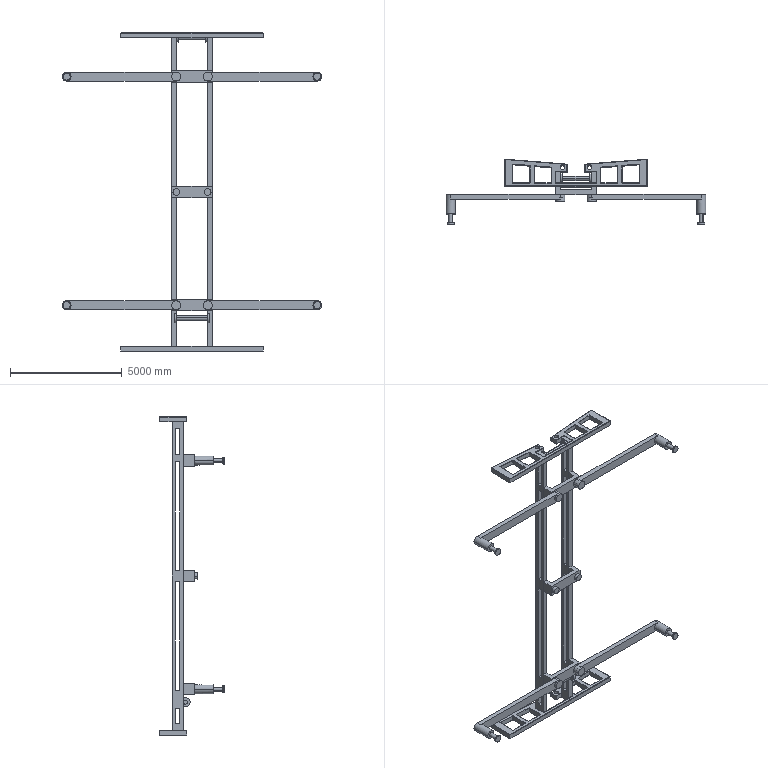Part | SolidWorks | features ReferencePattern 2, MirrorCompFeat 1 | 23 solids | 602 faces | box 11606 x 2886 x 14220 mm | volume 6344611681 mm3 | cylinder 266 | plane 224 | torus 88 | sphere 16 | cone 8 | commonest cylinder face diameters 20 x96 30 x58 175 x16 180 x16 275 x16 400 x16